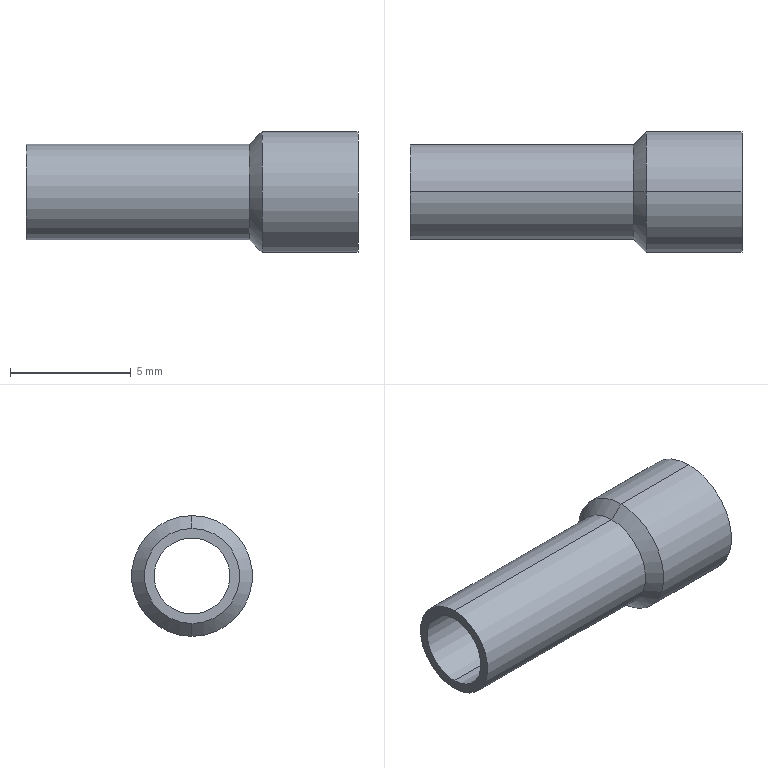Part | SolidWorks | features Revolution 1 | 1 solid | 14 faces | box 13.74 x 5 x 5 mm | volume 67.776 mm3 | cylinder 8 | cone 4 | plane 2 | commonest cylinder face diameters 3.14 x2 3.94 x2 4.2 x2 5 x2
STEP:
#1=CARTESIAN_POINT('',(9.406,0.,-1.57));
#2=VERTEX_POINT('',#1);
#3=CARTESIAN_POINT('',(9.406,0.,1.57));
#4=VERTEX_POINT('',#3);
#5=CARTESIAN_POINT('',(9.406,0.,0.));
#6=DIRECTION('',(-1.,0.,0.));
#7=DIRECTION('',(0.,0.,1.));
#8=AXIS2_PLACEMENT_3D('',#5,#6,#7);
#9=CIRCLE('',#8,1.57);
#10=EDGE_CURVE('',#2,#4,#9,.T.);
#11=ORIENTED_EDGE('',*,*,#10,.F.);
#12=CARTESIAN_POINT('',(0.,0.,-1.57));
#13=VERTEX_POINT('',#12);
#14=CARTESIAN_POINT('',(0.,0.,-1.57));
#15=DIRECTION('',(-1.,0.,0.));
#16=VECTOR('',#15,1000.);
#17=LINE('',#14,#16);
#18=EDGE_CURVE('',#2,#13,#17,.T.);
#19=ORIENTED_EDGE('',*,*,#18,.T.);
#20=CARTESIAN_POINT('',(0.,0.,1.57));
#21=VERTEX_POINT('',#20);
#22=CARTESIAN_POINT('',(0.,0.,0.));
#23=DIRECTION('',(-1.,0.,0.));
#24=DIRECTION('',(0.,0.,1.));
#25=AXIS2_PLACEMENT_3D('',#22,#23,#24);
#26=CIRCLE('',#25,1.57);
#27=EDGE_CURVE('',#13,#21,#26,.T.);
#28=ORIENTED_EDGE('',*,*,#27,.T.);
#29=CARTESIAN_POINT('',(0.,0.,1.57));
#30=DIRECTION('',(-1.,0.,0.));
#31=VECTOR('',#30,1000.);
#32=LINE('',#29,#31);
#33=EDGE_CURVE('',#4,#21,#32,.T.);
#34=ORIENTED_EDGE('',*,*,#33,.F.);
#35=EDGE_LOOP('',(#11,#19,#28,#34));
#36=FACE_OUTER_BOUND('',#35,.T.);
#37=CARTESIAN_POINT('',(0.,0.,0.));
#38=DIRECTION('',(-1.,0.,0.));
#39=DIRECTION('',(0.,0.,1.));
#40=AXIS2_PLACEMENT_3D('',#37,#38,#39);
#41=CYLINDRICAL_SURFACE('',#40,1.57);
#42=ADVANCED_FACE('',(#36),#41,.F.);
#43=ORIENTED_EDGE('',*,*,#10,.T.);
#44=CARTESIAN_POINT('',(9.936,0.,2.1));
#45=VERTEX_POINT('',#44);
#46=CARTESIAN_POINT('',(9.406,0.,1.57));
#47=DIRECTION('',(0.7071,0.,0.7071));
#48=VECTOR('',#47,1000.);
#49=LINE('',#46,#48);
#50=EDGE_CURVE('',#4,#45,#49,.T.);
#51=ORIENTED_EDGE('',*,*,#50,.T.);
#52=CARTESIAN_POINT('',(9.936,0.,-2.1));
#53=VERTEX_POINT('',#52);
#54=CARTESIAN_POINT('',(9.936,0.,0.));
#55=DIRECTION('',(-1.,0.,0.));
#56=DIRECTION('',(0.,0.,1.));
#57=AXIS2_PLACEMENT_3D('',#54,#55,#56);
#58=CIRCLE('',#57,2.1);
#59=EDGE_CURVE('',#53,#45,#58,.T.);
#60=ORIENTED_EDGE('',*,*,#59,.F.);
#61=CARTESIAN_POINT('',(9.406,0.,-1.57));
#62=DIRECTION('',(0.7071,0.,-0.7071));
#63=VECTOR('',#62,1000.);
#64=LINE('',#61,#63);
#65=EDGE_CURVE('',#2,#53,#64,.T.);
#66=ORIENTED_EDGE('',*,*,#65,.F.);
#67=EDGE_LOOP('',(#43,#51,#60,#66));
#68=FACE_OUTER_BOUND('',#67,.T.);
#69=CARTESIAN_POINT('',(9.406,0.,0.));
#70=DIRECTION('',(1.,0.,0.));
#71=DIRECTION('',(0.,0.,-1.));
#72=AXIS2_PLACEMENT_3D('',#69,#70,#71);
#73=CONICAL_SURFACE('',#72,1.57,0.7854);
#74=ADVANCED_FACE('',(#68),#73,.F.);
#75=CARTESIAN_POINT('',(13.74,0.,-2.1));
#76=VERTEX_POINT('',#75);
#77=CARTESIAN_POINT('',(13.74,0.,2.1));
#78=VERTEX_POINT('',#77);
#79=CARTESIAN_POINT('',(13.74,0.,0.));
#80=DIRECTION('',(-1.,0.,0.));
#81=DIRECTION('',(0.,0.,1.));
#82=AXIS2_PLACEMENT_3D('',#79,#80,#81);
#83=CIRCLE('',#82,2.1);
#84=EDGE_CURVE('',#76,#78,#83,.T.);
#85=ORIENTED_EDGE('',*,*,#84,.F.);
#86=CARTESIAN_POINT('',(0.,0.,-2.1));
#87=DIRECTION('',(-1.,0.,0.));
#88=VECTOR('',#87,1000.);
#89=LINE('',#86,#88);
#90=EDGE_CURVE('',#76,#53,#89,.T.);
#91=ORIENTED_EDGE('',*,*,#90,.T.);
#92=ORIENTED_EDGE('',*,*,#59,.T.);
#93=CARTESIAN_POINT('',(0.,0.,2.1));
#94=DIRECTION('',(-1.,0.,0.));
#95=VECTOR('',#94,1000.);
#96=LINE('',#93,#95);
#97=EDGE_CURVE('',#78,#45,#96,.T.);
#98=ORIENTED_EDGE('',*,*,#97,.F.);
#99=EDGE_LOOP('',(#85,#91,#92,#98));
#100=FACE_OUTER_BOUND('',#99,.T.);
#101=CARTESIAN_POINT('',(0.,0.,0.));
#102=DIRECTION('',(-1.,0.,0.));
#103=DIRECTION('',(0.,0.,1.));
#104=AXIS2_PLACEMENT_3D('',#101,#102,#103);
#105=CYLINDRICAL_SURFACE('',#104,2.1);
#106=ADVANCED_FACE('',(#100),#105,.F.);
#107=CARTESIAN_POINT('',(13.74,0.,2.5));
#108=VERTEX_POINT('',#107);
#109=CARTESIAN_POINT('',(13.74,0.,-2.5));
#110=VERTEX_POINT('',#109);
#111=CARTESIAN_POINT('',(13.74,0.,0.));
#112=DIRECTION('',(-1.,0.,0.));
#113=DIRECTION('',(0.,0.,1.));
#114=AXIS2_PLACEMENT_3D('',#111,#112,#113);
#115=CIRCLE('',#114,2.5);
#116=EDGE_CURVE('',#108,#110,#115,.T.);
#117=ORIENTED_EDGE('',*,*,#116,.T.);
#118=CARTESIAN_POINT('',(9.77,0.,-2.5));
#119=VERTEX_POINT('',#118);
#120=CARTESIAN_POINT('',(0.,0.,-2.5));
#121=DIRECTION('',(-1.,0.,0.));
#122=VECTOR('',#121,1000.);
#123=LINE('',#120,#122);
#124=EDGE_CURVE('',#110,#119,#123,.T.);
#125=ORIENTED_EDGE('',*,*,#124,.T.);
#126=CARTESIAN_POINT('',(9.77,0.,2.5));
#127=VERTEX_POINT('',#126);
#128=CARTESIAN_POINT('',(9.77,0.,0.));
#129=DIRECTION('',(-1.,0.,0.));
#130=DIRECTION('',(0.,0.,1.));
#131=AXIS2_PLACEMENT_3D('',#128,#129,#130);
#132=CIRCLE('',#131,2.5);
#133=EDGE_CURVE('',#127,#119,#132,.T.);
#134=ORIENTED_EDGE('',*,*,#133,.F.);
#135=CARTESIAN_POINT('',(0.,0.,2.5));
#136=DIRECTION('',(-1.,0.,0.));
#137=VECTOR('',#136,1000.);
#138=LINE('',#135,#137);
#139=EDGE_CURVE('',#108,#127,#138,.T.);
#140=ORIENTED_EDGE('',*,*,#139,.F.);
#141=EDGE_LOOP('',(#117,#125,#134,#140));
#142=FACE_OUTER_BOUND('',#141,.T.);
#143=CARTESIAN_POINT('',(0.,0.,0.));
#144=DIRECTION('',(-1.,0.,0.));
#145=DIRECTION('',(0.,0.,1.));
#146=AXIS2_PLACEMENT_3D('',#143,#144,#145);
#147=CYLINDRICAL_SURFACE('',#146,2.5);
#148=ADVANCED_FACE('',(#142),#147,.T.);
#149=CARTESIAN_POINT('',(9.24,0.,1.97));
#150=VERTEX_POINT('',#149);
#151=CARTESIAN_POINT('',(9.24,0.,-1.97));
#152=VERTEX_POINT('',#151);
#153=CARTESIAN_POINT('',(9.24,0.,0.));
#154=DIRECTION('',(-1.,0.,0.));
#155=DIRECTION('',(0.,0.,1.));
#156=AXIS2_PLACEMENT_3D('',#153,#154,#155);
#157=CIRCLE('',#156,1.97);
#158=EDGE_CURVE('',#150,#152,#157,.T.);
#159=ORIENTED_EDGE('',*,*,#158,.F.);
#160=CARTESIAN_POINT('',(9.77,0.,2.5));
#161=DIRECTION('',(0.7071,0.,0.7071));
#162=VECTOR('',#161,1000.);
#163=LINE('',#160,#162);
#164=EDGE_CURVE('',#150,#127,#163,.T.);
#165=ORIENTED_EDGE('',*,*,#164,.T.);
#166=ORIENTED_EDGE('',*,*,#133,.T.);
#167=CARTESIAN_POINT('',(9.77,0.,-2.5));
#168=DIRECTION('',(0.7071,0.,-0.7071));
#169=VECTOR('',#168,1000.);
#170=LINE('',#167,#169);
#171=EDGE_CURVE('',#152,#119,#170,.T.);
#172=ORIENTED_EDGE('',*,*,#171,.F.);
#173=EDGE_LOOP('',(#159,#165,#166,#172));
#174=FACE_OUTER_BOUND('',#173,.T.);
#175=CARTESIAN_POINT('',(9.77,0.,0.));
#176=DIRECTION('',(1.,0.,0.));
#177=DIRECTION('',(0.,0.,-1.));
#178=AXIS2_PLACEMENT_3D('',#175,#176,#177);
#179=CONICAL_SURFACE('',#178,2.5,0.7854);
#180=ADVANCED_FACE('',(#174),#179,.T.);
#181=ORIENTED_EDGE('',*,*,#158,.T.);
#182=CARTESIAN_POINT('',(0.,0.,-1.97));
#183=VERTEX_POINT('',#182);
#184=CARTESIAN_POINT('',(0.,0.,-1.97));
#185=DIRECTION('',(-1.,0.,0.));
#186=VECTOR('',#185,1000.);
#187=LINE('',#184,#186);
#188=EDGE_CURVE('',#152,#183,#187,.T.);
#189=ORIENTED_EDGE('',*,*,#188,.T.);
#190=CARTESIAN_POINT('',(0.,0.,1.97));
#191=VERTEX_POINT('',#190);
#192=CARTESIAN_POINT('',(0.,0.,0.));
#193=DIRECTION('',(-1.,0.,0.));
#194=DIRECTION('',(0.,0.,1.));
#195=AXIS2_PLACEMENT_3D('',#192,#193,#194);
#196=CIRCLE('',#195,1.97);
#197=EDGE_CURVE('',#191,#183,#196,.T.);
#198=ORIENTED_EDGE('',*,*,#197,.F.);
#199=CARTESIAN_POINT('',(0.,0.,1.97));
#200=DIRECTION('',(-1.,0.,0.));
#201=VECTOR('',#200,1000.);
#202=LINE('',#199,#201);
#203=EDGE_CURVE('',#150,#191,#202,.T.);
#204=ORIENTED_EDGE('',*,*,#203,.F.);
#205=EDGE_LOOP('',(#181,#189,#198,#204));
#206=FACE_OUTER_BOUND('',#205,.T.);
#207=CARTESIAN_POINT('',(0.,0.,0.));
#208=DIRECTION('',(-1.,0.,0.));
#209=DIRECTION('',(0.,0.,1.));
#210=AXIS2_PLACEMENT_3D('',#207,#208,#209);
#211=CYLINDRICAL_SURFACE('',#210,1.97);
#212=ADVANCED_FACE('',(#206),#211,.T.);
#213=CARTESIAN_POINT('',(0.,0.,0.));
#214=DIRECTION('',(-1.,0.,0.));
#215=DIRECTION('',(0.,0.,1.));
#216=AXIS2_PLACEMENT_3D('',#213,#214,#215);
#217=CIRCLE('',#216,1.57);
#218=EDGE_CURVE('',#21,#13,#217,.T.);
#219=ORIENTED_EDGE('',*,*,#218,.F.);
#220=ORIENTED_EDGE('',*,*,#27,.F.);
#221=EDGE_LOOP('',(#219,#220));
#222=FACE_BOUND('',#221,.T.);
#223=ORIENTED_EDGE('',*,*,#197,.T.);
#224=CARTESIAN_POINT('',(0.,0.,0.));
#225=DIRECTION('',(-1.,0.,0.));
#226=DIRECTION('',(0.,0.,1.));
#227=AXIS2_PLACEMENT_3D('',#224,#225,#226);
#228=CIRCLE('',#227,1.97);
#229=EDGE_CURVE('',#183,#191,#228,.T.);
#230=ORIENTED_EDGE('',*,*,#229,.T.);
#231=EDGE_LOOP('',(#223,#230));
#232=FACE_OUTER_BOUND('',#231,.T.);
#233=CARTESIAN_POINT('',(0.,1.57,0.));
#234=DIRECTION('',(1.,0.,0.));
#235=DIRECTION('',(0.,0.,-1.));
#236=AXIS2_PLACEMENT_3D('',#233,#234,#235);
#237=PLANE('',#236);
#238=ADVANCED_FACE('',(#222,#232),#237,.F.);
#239=ORIENTED_EDGE('',*,*,#188,.F.);
#240=CARTESIAN_POINT('',(9.24,0.,0.));
#241=DIRECTION('',(-1.,0.,0.));
#242=DIRECTION('',(0.,0.,1.));
#243=AXIS2_PLACEMENT_3D('',#240,#241,#242);
#244=CIRCLE('',#243,1.97);
#245=EDGE_CURVE('',#152,#150,#244,.T.);
#246=ORIENTED_EDGE('',*,*,#245,.T.);
#247=ORIENTED_EDGE('',*,*,#203,.T.);
#248=ORIENTED_EDGE('',*,*,#229,.F.);
#249=EDGE_LOOP('',(#239,#246,#247,#248));
#250=FACE_OUTER_BOUND('',#249,.T.);
#251=CARTESIAN_POINT('',(0.,0.,0.));
#252=DIRECTION('',(-1.,0.,0.));
#253=DIRECTION('',(0.,0.,1.));
#254=AXIS2_PLACEMENT_3D('',#251,#252,#253);
#255=CYLINDRICAL_SURFACE('',#254,1.97);
#256=ADVANCED_FACE('',(#250),#255,.T.);
#257=ORIENTED_EDGE('',*,*,#164,.F.);
#258=ORIENTED_EDGE('',*,*,#245,.F.);
#259=ORIENTED_EDGE('',*,*,#171,.T.);
#260=CARTESIAN_POINT('',(9.77,0.,0.));
#261=DIRECTION('',(-1.,0.,0.));
#262=DIRECTION('',(0.,0.,1.));
#263=AXIS2_PLACEMENT_3D('',#260,#261,#262);
#264=CIRCLE('',#263,2.5);
#265=EDGE_CURVE('',#119,#127,#264,.T.);
#266=ORIENTED_EDGE('',*,*,#265,.T.);
#267=EDGE_LOOP('',(#257,#258,#259,#266));
#268=FACE_OUTER_BOUND('',#267,.T.);
#269=CARTESIAN_POINT('',(9.77,0.,0.));
#270=DIRECTION('',(1.,0.,0.));
#271=DIRECTION('',(0.,0.,-1.));
#272=AXIS2_PLACEMENT_3D('',#269,#270,#271);
#273=CONICAL_SURFACE('',#272,2.5,0.7854);
#274=ADVANCED_FACE('',(#268),#273,.T.);
#275=ORIENTED_EDGE('',*,*,#124,.F.);
#276=CARTESIAN_POINT('',(13.74,0.,0.));
#277=DIRECTION('',(-1.,0.,0.));
#278=DIRECTION('',(0.,0.,1.));
#279=AXIS2_PLACEMENT_3D('',#276,#277,#278);
#280=CIRCLE('',#279,2.5);
#281=EDGE_CURVE('',#110,#108,#280,.T.);
#282=ORIENTED_EDGE('',*,*,#281,.T.);
#283=ORIENTED_EDGE('',*,*,#139,.T.);
#284=ORIENTED_EDGE('',*,*,#265,.F.);
#285=EDGE_LOOP('',(#275,#282,#283,#284));
#286=FACE_OUTER_BOUND('',#285,.T.);
#287=CARTESIAN_POINT('',(0.,0.,0.));
#288=DIRECTION('',(-1.,0.,0.));
#289=DIRECTION('',(0.,0.,1.));
#290=AXIS2_PLACEMENT_3D('',#287,#288,#289);
#291=CYLINDRICAL_SURFACE('',#290,2.5);
#292=ADVANCED_FACE('',(#286),#291,.T.);
#293=ORIENTED_EDGE('',*,*,#116,.F.);
#294=ORIENTED_EDGE('',*,*,#281,.F.);
#295=EDGE_LOOP('',(#293,#294));
#296=FACE_OUTER_BOUND('',#295,.T.);
#297=CARTESIAN_POINT('',(13.74,0.,0.));
#298=DIRECTION('',(-1.,0.,0.));
#299=DIRECTION('',(0.,0.,1.));
#300=AXIS2_PLACEMENT_3D('',#297,#298,#299);
#301=CIRCLE('',#300,2.1);
#302=EDGE_CURVE('',#78,#76,#301,.T.);
#303=ORIENTED_EDGE('',*,*,#302,.T.);
#304=ORIENTED_EDGE('',*,*,#84,.T.);
#305=EDGE_LOOP('',(#303,#304));
#306=FACE_BOUND('',#305,.T.);
#307=CARTESIAN_POINT('',(13.74,2.1,0.));
#308=DIRECTION('',(-1.,0.,0.));
#309=DIRECTION('',(0.,0.,1.));
#310=AXIS2_PLACEMENT_3D('',#307,#308,#309);
#311=PLANE('',#310);
#312=ADVANCED_FACE('',(#296,#306),#311,.F.);
#313=ORIENTED_EDGE('',*,*,#90,.F.);
#314=ORIENTED_EDGE('',*,*,#302,.F.);
#315=ORIENTED_EDGE('',*,*,#97,.T.);
#316=CARTESIAN_POINT('',(9.936,0.,0.));
#317=DIRECTION('',(-1.,0.,0.));
#318=DIRECTION('',(0.,0.,1.));
#319=AXIS2_PLACEMENT_3D('',#316,#317,#318);
#320=CIRCLE('',#319,2.1);
#321=EDGE_CURVE('',#45,#53,#320,.T.);
#322=ORIENTED_EDGE('',*,*,#321,.T.);
#323=EDGE_LOOP('',(#313,#314,#315,#322));
#324=FACE_OUTER_BOUND('',#323,.T.);
#325=CARTESIAN_POINT('',(0.,0.,0.));
#326=DIRECTION('',(-1.,0.,0.));
#327=DIRECTION('',(0.,0.,1.));
#328=AXIS2_PLACEMENT_3D('',#325,#326,#327);
#329=CYLINDRICAL_SURFACE('',#328,2.1);
#330=ADVANCED_FACE('',(#324),#329,.F.);
#331=ORIENTED_EDGE('',*,*,#50,.F.);
#332=CARTESIAN_POINT('',(9.406,0.,0.));
#333=DIRECTION('',(-1.,0.,0.));
#334=DIRECTION('',(0.,0.,1.));
#335=AXIS2_PLACEMENT_3D('',#332,#333,#334);
#336=CIRCLE('',#335,1.57);
#337=EDGE_CURVE('',#4,#2,#336,.T.);
#338=ORIENTED_EDGE('',*,*,#337,.T.);
#339=ORIENTED_EDGE('',*,*,#65,.T.);
#340=ORIENTED_EDGE('',*,*,#321,.F.);
#341=EDGE_LOOP('',(#331,#338,#339,#340));
#342=FACE_OUTER_BOUND('',#341,.T.);
#343=CARTESIAN_POINT('',(9.406,0.,0.));
#344=DIRECTION('',(1.,0.,0.));
#345=DIRECTION('',(0.,0.,-1.));
#346=AXIS2_PLACEMENT_3D('',#343,#344,#345);
#347=CONICAL_SURFACE('',#346,1.57,0.7854);
#348=ADVANCED_FACE('',(#342),#347,.F.);
#349=ORIENTED_EDGE('',*,*,#18,.F.);
#350=ORIENTED_EDGE('',*,*,#337,.F.);
#351=ORIENTED_EDGE('',*,*,#33,.T.);
#352=ORIENTED_EDGE('',*,*,#218,.T.);
#353=EDGE_LOOP('',(#349,#350,#351,#352));
#354=FACE_OUTER_BOUND('',#353,.T.);
#355=CARTESIAN_POINT('',(0.,0.,0.));
#356=DIRECTION('',(-1.,0.,0.));
#357=DIRECTION('',(0.,0.,1.));
#358=AXIS2_PLACEMENT_3D('',#355,#356,#357);
#359=CYLINDRICAL_SURFACE('',#358,1.57);
#360=ADVANCED_FACE('',(#354),#359,.F.);
#361=CLOSED_SHELL('',(#42,#74,#106,#148,#180,#212,#238,#256,#274,#292,#312,#330,#348,#360));
#362=MANIFOLD_SOLID_BREP('',#361);
#363=CARTESIAN_POINT('',(0.,0.,0.));
#364=DIRECTION('',(0.,0.,1.));
#365=DIRECTION('',(1.,0.,0.));
#366=AXIS2_PLACEMENT_3D('',#363,#364,#365);
#367=(LENGTH_UNIT()NAMED_UNIT(*)SI_UNIT(.MILLI.,.METRE.));
#368=UNCERTAINTY_MEASURE_WITH_UNIT(LENGTH_MEASURE(0.00001),#367,'','');
#369=(NAMED_UNIT(*)PLANE_ANGLE_UNIT()SI_UNIT($,.RADIAN.));
#370=(NAMED_UNIT(*)SI_UNIT($,.STERADIAN.)SOLID_ANGLE_UNIT());
#371=(GEOMETRIC_REPRESENTATION_CONTEXT(3)GLOBAL_UNCERTAINTY_ASSIGNED_CONTEXT((#368))GLOBAL_UNIT_ASSIGNED_CONTEXT((#367,#369,#370))REPRESENTATION_CONTEXT('',''));
#372=ADVANCED_BREP_SHAPE_REPRESENTATION('',(#362,#366),#371);